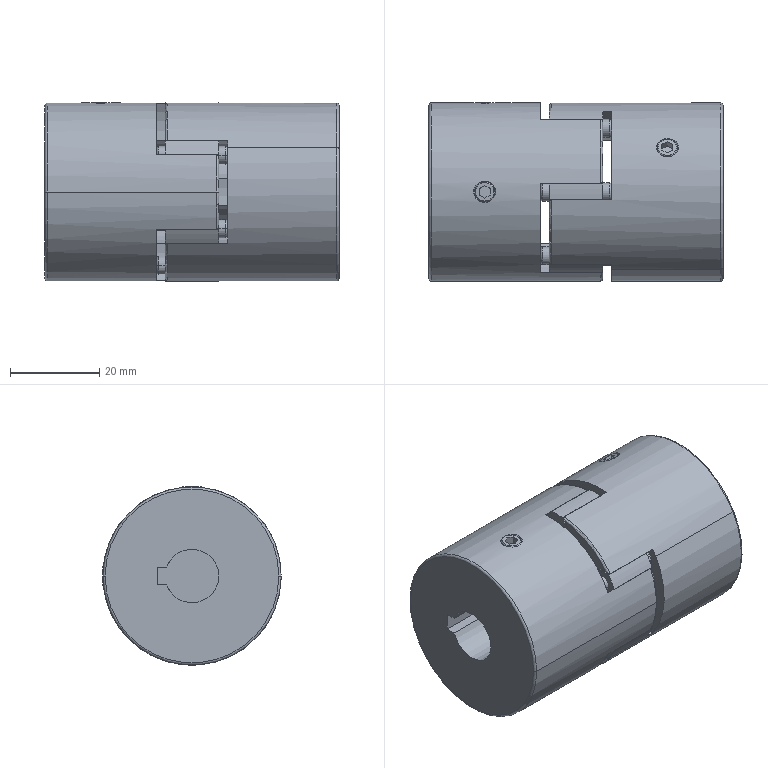Part | SolidWorks | features BaseBody 3 | 3 solids | 231 faces | box 66 x 40 x 40 mm | volume 67909 mm3 | cylinder 86 | plane 68 | torus 49 | cone 28 | commonest cylinder face diameters 23 x27 4 x18 40 x10 4.134 x8 22.8 x7 24 x7